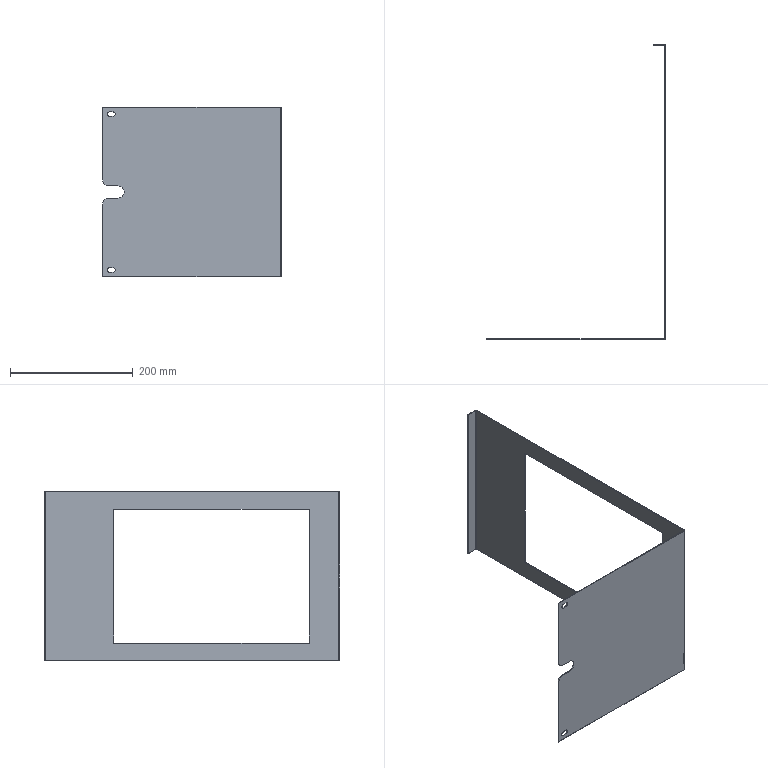Part | SolidWorks | features ICE 2, Cut 1, EdgeFlange 1, Fillet 1, FlatPattern 1, LPattern 1, SMBaseFlange 1, SheetMetal 1 | 1 solid | 40 faces | box 291.5 x 482 x 276.8 mm | volume 222164 mm3 | plane 29 | cylinder 11 | commonest cylinder face diameters 7 x4 20 x3 0.4 x2 3.4 x2
STEP:
#1=CARTESIAN_POINT('',(0.,0.,138.4));
#2=VERTEX_POINT('',#1);
#3=CARTESIAN_POINT('',(0.,0.,20.));
#4=VERTEX_POINT('',#3);
#5=CARTESIAN_POINT('',(0.,0.,138.4));
#6=DIRECTION('',(0.,0.,-1.));
#7=VECTOR('',#6,1000.);
#8=LINE('',#5,#7);
#9=EDGE_CURVE('',#2,#4,#8,.T.);
#10=ORIENTED_EDGE('',*,*,#9,.T.);
#11=CARTESIAN_POINT('',(0.,-1.5,20.));
#12=VERTEX_POINT('',#11);
#13=CARTESIAN_POINT('',(0.,-1.5,20.));
#14=DIRECTION('',(0.,-1.,0.));
#15=VECTOR('',#14,1000.);
#16=LINE('',#13,#15);
#17=EDGE_CURVE('',#4,#12,#16,.T.);
#18=ORIENTED_EDGE('',*,*,#17,.T.);
#19=CARTESIAN_POINT('',(0.,-1.5,138.4));
#20=VERTEX_POINT('',#19);
#21=CARTESIAN_POINT('',(0.,-1.5,138.4));
#22=DIRECTION('',(0.,0.,-1.));
#23=VECTOR('',#22,1000.);
#24=LINE('',#21,#23);
#25=EDGE_CURVE('',#20,#12,#24,.T.);
#26=ORIENTED_EDGE('',*,*,#25,.F.);
#27=CARTESIAN_POINT('',(0.,-1.5,138.4));
#28=DIRECTION('',(0.,1.,0.));
#29=VECTOR('',#28,1000.);
#30=LINE('',#27,#29);
#31=EDGE_CURVE('',#20,#2,#30,.T.);
#32=ORIENTED_EDGE('',*,*,#31,.T.);
#33=EDGE_LOOP('',(#10,#18,#26,#32));
#34=FACE_OUTER_BOUND('',#33,.T.);
#35=CARTESIAN_POINT('',(0.,-1.5,138.4));
#36=DIRECTION('',(-1.,0.,0.));
#37=DIRECTION('',(0.,0.,1.));
#38=AXIS2_PLACEMENT_3D('',#35,#36,#37);
#39=PLANE('',#38);
#40=ADVANCED_FACE('',(#34),#39,.T.);
#41=CARTESIAN_POINT('',(291.5,48.5,109.15));
#42=VERTEX_POINT('',#41);
#43=CARTESIAN_POINT('',(291.5,48.5,-109.35));
#44=VERTEX_POINT('',#43);
#45=CARTESIAN_POINT('',(291.5,48.5,109.15));
#46=DIRECTION('',(0.,0.,-1.));
#47=VECTOR('',#46,1000.);
#48=LINE('',#45,#47);
#49=EDGE_CURVE('',#42,#44,#48,.T.);
#50=ORIENTED_EDGE('',*,*,#49,.F.);
#51=CARTESIAN_POINT('',(291.5,367.1,109.15));
#52=VERTEX_POINT('',#51);
#53=CARTESIAN_POINT('',(291.5,367.1,109.15));
#54=DIRECTION('',(0.,-1.,0.));
#55=VECTOR('',#54,1000.);
#56=LINE('',#53,#55);
#57=EDGE_CURVE('',#52,#42,#56,.T.);
#58=ORIENTED_EDGE('',*,*,#57,.F.);
#59=CARTESIAN_POINT('',(291.5,367.1,-109.35));
#60=VERTEX_POINT('',#59);
#61=CARTESIAN_POINT('',(291.5,367.1,109.15));
#62=DIRECTION('',(0.,0.,1.));
#63=VECTOR('',#62,1000.);
#64=LINE('',#61,#63);
#65=EDGE_CURVE('',#60,#52,#64,.T.);
#66=ORIENTED_EDGE('',*,*,#65,.F.);
#67=CARTESIAN_POINT('',(291.5,367.1,-109.35));
#68=DIRECTION('',(0.,1.,0.));
#69=VECTOR('',#68,1000.);
#70=LINE('',#67,#69);
#71=EDGE_CURVE('',#44,#60,#70,.T.);
#72=ORIENTED_EDGE('',*,*,#71,.F.);
#73=EDGE_LOOP('',(#50,#58,#66,#72));
#74=FACE_BOUND('',#73,.T.);
#75=CARTESIAN_POINT('',(291.5,478.8,-138.4));
#76=VERTEX_POINT('',#75);
#77=CARTESIAN_POINT('',(291.5,478.8,138.4));
#78=VERTEX_POINT('',#77);
#79=CARTESIAN_POINT('',(291.5,478.8,-138.4));
#80=DIRECTION('',(0.,0.,1.));
#81=VECTOR('',#80,1000.);
#82=LINE('',#79,#81);
#83=EDGE_CURVE('',#76,#78,#82,.T.);
#84=ORIENTED_EDGE('',*,*,#83,.T.);
#85=CARTESIAN_POINT('',(291.5,0.2,138.4));
#86=VERTEX_POINT('',#85);
#87=CARTESIAN_POINT('',(291.5,0.,138.4));
#88=DIRECTION('',(0.,1.,0.));
#89=VECTOR('',#88,1000.);
#90=LINE('',#87,#89);
#91=EDGE_CURVE('',#86,#78,#90,.T.);
#92=ORIENTED_EDGE('',*,*,#91,.F.);
#93=CARTESIAN_POINT('',(291.5,0.2,-138.4));
#94=VERTEX_POINT('',#93);
#95=CARTESIAN_POINT('',(291.5,0.2,138.4));
#96=DIRECTION('',(0.,0.,-1.));
#97=VECTOR('',#96,1000.);
#98=LINE('',#95,#97);
#99=EDGE_CURVE('',#86,#94,#98,.T.);
#100=ORIENTED_EDGE('',*,*,#99,.T.);
#101=CARTESIAN_POINT('',(291.5,0.,-138.4));
#102=DIRECTION('',(0.,1.,0.));
#103=VECTOR('',#102,1000.);
#104=LINE('',#101,#103);
#105=EDGE_CURVE('',#94,#76,#104,.T.);
#106=ORIENTED_EDGE('',*,*,#105,.T.);
#107=EDGE_LOOP('',(#84,#92,#100,#106));
#108=FACE_OUTER_BOUND('',#107,.T.);
#109=CARTESIAN_POINT('',(291.5,0.,138.4));
#110=DIRECTION('',(-1.,0.,0.));
#111=DIRECTION('',(0.,0.,1.));
#112=AXIS2_PLACEMENT_3D('',#109,#110,#111);
#113=PLANE('',#112);
#114=ADVANCED_FACE('',(#74,#108),#113,.F.);
#115=CARTESIAN_POINT('',(290.,367.1,109.15));
#116=VERTEX_POINT('',#115);
#117=CARTESIAN_POINT('',(290.,48.5,109.15));
#118=VERTEX_POINT('',#117);
#119=CARTESIAN_POINT('',(290.,367.1,109.15));
#120=DIRECTION('',(0.,-1.,0.));
#121=VECTOR('',#120,1000.);
#122=LINE('',#119,#121);
#123=EDGE_CURVE('',#116,#118,#122,.T.);
#124=ORIENTED_EDGE('',*,*,#123,.T.);
#125=CARTESIAN_POINT('',(290.,48.5,-109.35));
#126=VERTEX_POINT('',#125);
#127=CARTESIAN_POINT('',(290.,48.5,109.15));
#128=DIRECTION('',(0.,0.,-1.));
#129=VECTOR('',#128,1000.);
#130=LINE('',#127,#129);
#131=EDGE_CURVE('',#118,#126,#130,.T.);
#132=ORIENTED_EDGE('',*,*,#131,.T.);
#133=CARTESIAN_POINT('',(290.,367.1,-109.35));
#134=VERTEX_POINT('',#133);
#135=CARTESIAN_POINT('',(290.,367.1,-109.35));
#136=DIRECTION('',(0.,1.,0.));
#137=VECTOR('',#136,1000.);
#138=LINE('',#135,#137);
#139=EDGE_CURVE('',#126,#134,#138,.T.);
#140=ORIENTED_EDGE('',*,*,#139,.T.);
#141=CARTESIAN_POINT('',(290.,367.1,109.15));
#142=DIRECTION('',(0.,0.,1.));
#143=VECTOR('',#142,1000.);
#144=LINE('',#141,#143);
#145=EDGE_CURVE('',#134,#116,#144,.T.);
#146=ORIENTED_EDGE('',*,*,#145,.T.);
#147=EDGE_LOOP('',(#124,#132,#140,#146));
#148=FACE_BOUND('',#147,.T.);
#149=CARTESIAN_POINT('',(290.,0.2,138.4));
#150=VERTEX_POINT('',#149);
#151=CARTESIAN_POINT('',(290.,478.8,138.4));
#152=VERTEX_POINT('',#151);
#153=CARTESIAN_POINT('',(290.,0.,138.4));
#154=DIRECTION('',(0.,1.,0.));
#155=VECTOR('',#154,1000.);
#156=LINE('',#153,#155);
#157=EDGE_CURVE('',#150,#152,#156,.T.);
#158=ORIENTED_EDGE('',*,*,#157,.T.);
#159=CARTESIAN_POINT('',(290.,478.8,-138.4));
#160=VERTEX_POINT('',#159);
#161=CARTESIAN_POINT('',(290.,478.8,-138.4));
#162=DIRECTION('',(0.,0.,1.));
#163=VECTOR('',#162,1000.);
#164=LINE('',#161,#163);
#165=EDGE_CURVE('',#160,#152,#164,.T.);
#166=ORIENTED_EDGE('',*,*,#165,.F.);
#167=CARTESIAN_POINT('',(290.,0.2,-138.4));
#168=VERTEX_POINT('',#167);
#169=CARTESIAN_POINT('',(290.,0.,-138.4));
#170=DIRECTION('',(0.,1.,0.));
#171=VECTOR('',#170,1000.);
#172=LINE('',#169,#171);
#173=EDGE_CURVE('',#168,#160,#172,.T.);
#174=ORIENTED_EDGE('',*,*,#173,.F.);
#175=CARTESIAN_POINT('',(290.,0.2,138.4));
#176=DIRECTION('',(0.,0.,-1.));
#177=VECTOR('',#176,1000.);
#178=LINE('',#175,#177);
#179=EDGE_CURVE('',#150,#168,#178,.T.);
#180=ORIENTED_EDGE('',*,*,#179,.F.);
#181=EDGE_LOOP('',(#158,#166,#174,#180));
#182=FACE_OUTER_BOUND('',#181,.T.);
#183=CARTESIAN_POINT('',(290.,0.,138.4));
#184=DIRECTION('',(-1.,0.,0.));
#185=DIRECTION('',(0.,0.,1.));
#186=AXIS2_PLACEMENT_3D('',#183,#184,#185);
#187=PLANE('',#186);
#188=ADVANCED_FACE('',(#148,#182),#187,.T.);
#189=ORIENTED_EDGE('',*,*,#173,.T.);
#190=CARTESIAN_POINT('',(290.,478.8,-138.4));
#191=DIRECTION('',(1.,0.,0.));
#192=VECTOR('',#191,1000.);
#193=LINE('',#190,#192);
#194=EDGE_CURVE('',#160,#76,#193,.T.);
#195=ORIENTED_EDGE('',*,*,#194,.T.);
#196=ORIENTED_EDGE('',*,*,#105,.F.);
#197=CARTESIAN_POINT('',(291.5,0.2,-138.4));
#198=DIRECTION('',(-1.,0.,0.));
#199=VECTOR('',#198,1000.);
#200=LINE('',#197,#199);
#201=EDGE_CURVE('',#94,#168,#200,.T.);
#202=ORIENTED_EDGE('',*,*,#201,.T.);
#203=EDGE_LOOP('',(#189,#195,#196,#202));
#204=FACE_OUTER_BOUND('',#203,.T.);
#205=CARTESIAN_POINT('',(289.8,0.2,-138.4));
#206=DIRECTION('',(0.,0.,-1.));
#207=DIRECTION('',(-1.,0.,0.));
#208=AXIS2_PLACEMENT_3D('',#205,#206,#207);
#209=PLANE('',#208);
#210=ADVANCED_FACE('',(#204),#209,.T.);
#211=CARTESIAN_POINT('',(290.,0.2,138.4));
#212=DIRECTION('',(1.,0.,0.));
#213=VECTOR('',#212,1000.);
#214=LINE('',#211,#213);
#215=EDGE_CURVE('',#150,#86,#214,.T.);
#216=ORIENTED_EDGE('',*,*,#215,.F.);
#217=CARTESIAN_POINT('',(289.8,0.,138.4));
#218=VERTEX_POINT('',#217);
#219=CARTESIAN_POINT('',(289.8,0.2,138.4));
#220=DIRECTION('',(0.,0.,1.));
#221=DIRECTION('',(-1.,0.,0.));
#222=AXIS2_PLACEMENT_3D('',#219,#220,#221);
#223=CIRCLE('',#222,0.2);
#224=EDGE_CURVE('',#218,#150,#223,.T.);
#225=ORIENTED_EDGE('',*,*,#224,.F.);
#226=CARTESIAN_POINT('',(289.8,-1.5,138.4));
#227=VERTEX_POINT('',#226);
#228=CARTESIAN_POINT('',(289.8,-1.5,138.4));
#229=DIRECTION('',(0.,1.,0.));
#230=VECTOR('',#229,1000.);
#231=LINE('',#228,#230);
#232=EDGE_CURVE('',#227,#218,#231,.T.);
#233=ORIENTED_EDGE('',*,*,#232,.F.);
#234=CARTESIAN_POINT('',(289.8,0.2,138.4));
#235=DIRECTION('',(0.,0.,1.));
#236=DIRECTION('',(1.,0.,0.));
#237=AXIS2_PLACEMENT_3D('',#234,#235,#236);
#238=CIRCLE('',#237,1.7);
#239=EDGE_CURVE('',#227,#86,#238,.T.);
#240=ORIENTED_EDGE('',*,*,#239,.T.);
#241=EDGE_LOOP('',(#216,#225,#233,#240));
#242=FACE_OUTER_BOUND('',#241,.T.);
#243=CARTESIAN_POINT('',(290.,0.2,138.4));
#244=DIRECTION('',(0.,0.,1.));
#245=DIRECTION('',(1.,0.,0.));
#246=AXIS2_PLACEMENT_3D('',#243,#244,#245);
#247=PLANE('',#246);
#248=ADVANCED_FACE('',(#242),#247,.T.);
#249=CARTESIAN_POINT('',(290.,478.8,138.4));
#250=DIRECTION('',(1.,0.,0.));
#251=VECTOR('',#250,1000.);
#252=LINE('',#249,#251);
#253=EDGE_CURVE('',#152,#78,#252,.T.);
#254=ORIENTED_EDGE('',*,*,#253,.F.);
#255=ORIENTED_EDGE('',*,*,#157,.F.);
#256=ORIENTED_EDGE('',*,*,#215,.T.);
#257=ORIENTED_EDGE('',*,*,#91,.T.);
#258=EDGE_LOOP('',(#254,#255,#256,#257));
#259=FACE_OUTER_BOUND('',#258,.T.);
#260=CARTESIAN_POINT('',(289.8,-1.5,138.4));
#261=DIRECTION('',(0.,0.,1.));
#262=DIRECTION('',(1.,0.,0.));
#263=AXIS2_PLACEMENT_3D('',#260,#261,#262);
#264=PLANE('',#263);
#265=ADVANCED_FACE('',(#259),#264,.T.);
#266=CARTESIAN_POINT('',(289.8,0.,-138.4));
#267=VERTEX_POINT('',#266);
#268=CARTESIAN_POINT('',(289.8,-1.5,-138.4));
#269=VERTEX_POINT('',#268);
#270=CARTESIAN_POINT('',(289.8,0.,-138.4));
#271=DIRECTION('',(0.,-1.,0.));
#272=VECTOR('',#271,1000.);
#273=LINE('',#270,#272);
#274=EDGE_CURVE('',#267,#269,#273,.T.);
#275=ORIENTED_EDGE('',*,*,#274,.F.);
#276=CARTESIAN_POINT('',(289.8,0.2,-138.4));
#277=DIRECTION('',(0.,0.,1.));
#278=DIRECTION('',(-1.,0.,0.));
#279=AXIS2_PLACEMENT_3D('',#276,#277,#278);
#280=CIRCLE('',#279,0.2);
#281=EDGE_CURVE('',#267,#168,#280,.T.);
#282=ORIENTED_EDGE('',*,*,#281,.T.);
#283=ORIENTED_EDGE('',*,*,#201,.F.);
#284=CARTESIAN_POINT('',(289.8,0.2,-138.4));
#285=DIRECTION('',(0.,0.,1.));
#286=DIRECTION('',(1.,0.,0.));
#287=AXIS2_PLACEMENT_3D('',#284,#285,#286);
#288=CIRCLE('',#287,1.7);
#289=EDGE_CURVE('',#269,#94,#288,.T.);
#290=ORIENTED_EDGE('',*,*,#289,.F.);
#291=EDGE_LOOP('',(#275,#282,#283,#290));
#292=FACE_OUTER_BOUND('',#291,.T.);
#293=CARTESIAN_POINT('',(289.8,0.,-138.4));
#294=DIRECTION('',(0.,0.,-1.));
#295=DIRECTION('',(-1.,0.,0.));
#296=AXIS2_PLACEMENT_3D('',#293,#294,#295);
#297=PLANE('',#296);
#298=ADVANCED_FACE('',(#292),#297,.T.);
#299=CARTESIAN_POINT('',(0.,0.,-138.4));
#300=VERTEX_POINT('',#299);
#301=CARTESIAN_POINT('',(0.,0.,-138.4));
#302=DIRECTION('',(1.,0.,0.));
#303=VECTOR('',#302,1000.);
#304=LINE('',#301,#303);
#305=EDGE_CURVE('',#300,#267,#304,.T.);
#306=ORIENTED_EDGE('',*,*,#305,.T.);
#307=ORIENTED_EDGE('',*,*,#274,.T.);
#308=CARTESIAN_POINT('',(0.,-1.5,-138.4));
#309=VERTEX_POINT('',#308);
#310=CARTESIAN_POINT('',(0.,-1.5,-138.4));
#311=DIRECTION('',(1.,0.,0.));
#312=VECTOR('',#311,1000.);
#313=LINE('',#310,#312);
#314=EDGE_CURVE('',#309,#269,#313,.T.);
#315=ORIENTED_EDGE('',*,*,#314,.F.);
#316=CARTESIAN_POINT('',(0.,-1.5,-138.4));
#317=DIRECTION('',(0.,1.,0.));
#318=VECTOR('',#317,1000.);
#319=LINE('',#316,#318);
#320=EDGE_CURVE('',#309,#300,#319,.T.);
#321=ORIENTED_EDGE('',*,*,#320,.T.);
#322=EDGE_LOOP('',(#306,#307,#315,#321));
#323=FACE_OUTER_BOUND('',#322,.T.);
#324=CARTESIAN_POINT('',(291.5,0.2,-138.4));
#325=DIRECTION('',(0.,0.,-1.));
#326=DIRECTION('',(-1.,0.,0.));
#327=AXIS2_PLACEMENT_3D('',#324,#325,#326);
#328=PLANE('',#327);
#329=ADVANCED_FACE('',(#323),#328,.T.);
#330=ORIENTED_EDGE('',*,*,#281,.F.);
#331=CARTESIAN_POINT('',(289.8,0.,138.4));
#332=DIRECTION('',(0.,0.,-1.));
#333=VECTOR('',#332,1000.);
#334=LINE('',#331,#333);
#335=EDGE_CURVE('',#218,#267,#334,.T.);
#336=ORIENTED_EDGE('',*,*,#335,.F.);
#337=ORIENTED_EDGE('',*,*,#224,.T.);
#338=ORIENTED_EDGE('',*,*,#179,.T.);
#339=EDGE_LOOP('',(#330,#336,#337,#338));
#340=FACE_OUTER_BOUND('',#339,.T.);
#341=CARTESIAN_POINT('',(289.8,0.2,138.4));
#342=DIRECTION('',(0.,0.,-1.));
#343=DIRECTION('',(-1.,0.,0.));
#344=AXIS2_PLACEMENT_3D('',#341,#342,#343);
#345=CYLINDRICAL_SURFACE('',#344,0.2);
#346=ADVANCED_FACE('',(#340),#345,.F.);
#347=CARTESIAN_POINT('',(10.,0.,10.));
#348=VERTEX_POINT('',#347);
#349=CARTESIAN_POINT('',(25.,0.,10.));
#350=VERTEX_POINT('',#349);
#351=CARTESIAN_POINT('',(25.,0.,10.));
#352=DIRECTION('',(1.,0.,0.));
#353=VECTOR('',#352,1000.);
#354=LINE('',#351,#353);
#355=EDGE_CURVE('',#348,#350,#354,.T.);
#356=ORIENTED_EDGE('',*,*,#355,.F.);
#357=CARTESIAN_POINT('',(10.,0.,20.));
#358=DIRECTION('',(0.,1.,0.));
#359=DIRECTION('',(0.,0.,1.));
#360=AXIS2_PLACEMENT_3D('',#357,#358,#359);
#361=CIRCLE('',#360,10.);
#362=EDGE_CURVE('',#348,#4,#361,.T.);
#363=ORIENTED_EDGE('',*,*,#362,.T.);
#364=ORIENTED_EDGE('',*,*,#9,.F.);
#365=CARTESIAN_POINT('',(0.,0.,138.4));
#366=DIRECTION('',(1.,0.,0.));
#367=VECTOR('',#366,1000.);
#368=LINE('',#365,#367);
#369=EDGE_CURVE('',#2,#218,#368,.T.);
#370=ORIENTED_EDGE('',*,*,#369,.T.);
#371=ORIENTED_EDGE('',*,*,#335,.T.);
#372=ORIENTED_EDGE('',*,*,#305,.F.);
#373=CARTESIAN_POINT('',(0.,0.,-20.));
#374=VERTEX_POINT('',#373);
#375=CARTESIAN_POINT('',(0.,0.,138.4));
#376=DIRECTION('',(0.,0.,-1.));
#377=VECTOR('',#376,1000.);
#378=LINE('',#375,#377);
#379=EDGE_CURVE('',#374,#300,#378,.T.);
#380=ORIENTED_EDGE('',*,*,#379,.F.);
#381=CARTESIAN_POINT('',(10.,0.,-10.));
#382=VERTEX_POINT('',#381);
#383=CARTESIAN_POINT('',(10.,0.,-20.));
#384=DIRECTION('',(0.,1.,0.));
#385=DIRECTION('',(0.,0.,1.));
#386=AXIS2_PLACEMENT_3D('',#383,#384,#385);
#387=CIRCLE('',#386,10.);
#388=EDGE_CURVE('',#374,#382,#387,.T.);
#389=ORIENTED_EDGE('',*,*,#388,.T.);
#390=CARTESIAN_POINT('',(25.,0.,-10.));
#391=VERTEX_POINT('',#390);
#392=CARTESIAN_POINT('',(25.,0.,-10.));
#393=DIRECTION('',(-1.,0.,0.));
#394=VECTOR('',#393,1000.);
#395=LINE('',#392,#394);
#396=EDGE_CURVE('',#391,#382,#395,.T.);
#397=ORIENTED_EDGE('',*,*,#396,.F.);
#398=CARTESIAN_POINT('',(25.,0.,0.));
#399=DIRECTION('',(0.,1.,0.));
#400=DIRECTION('',(0.,0.,1.));
#401=AXIS2_PLACEMENT_3D('',#398,#399,#400);
#402=CIRCLE('',#401,10.);
#403=EDGE_CURVE('',#350,#391,#402,.T.);
#404=ORIENTED_EDGE('',*,*,#403,.F.);
#405=EDGE_LOOP('',(#356,#363,#364,#370,#371,#372,#380,#389,#397,#404));
#406=FACE_OUTER_BOUND('',#405,.T.);
#407=CARTESIAN_POINT('',(11.,0.,-130.75));
#408=VERTEX_POINT('',#407);
#409=CARTESIAN_POINT('',(11.,0.,-123.75));
#410=VERTEX_POINT('',#409);
#411=CARTESIAN_POINT('',(11.,0.,-127.25));
#412=DIRECTION('',(0.,1.,0.));
#413=DIRECTION('',(0.,0.,1.));
#414=AXIS2_PLACEMENT_3D('',#411,#412,#413);
#415=CIRCLE('',#414,3.5);
#416=EDGE_CURVE('',#408,#410,#415,.T.);
#417=ORIENTED_EDGE('',*,*,#416,.F.);
#418=CARTESIAN_POINT('',(17.,0.,-130.75));
#419=VERTEX_POINT('',#418);
#420=CARTESIAN_POINT('',(11.,0.,-130.75));
#421=DIRECTION('',(-1.,0.,0.));
#422=VECTOR('',#421,1000.);
#423=LINE('',#420,#422);
#424=EDGE_CURVE('',#419,#408,#423,.T.);
#425=ORIENTED_EDGE('',*,*,#424,.F.);
#426=CARTESIAN_POINT('',(17.,0.,-123.75));
#427=VERTEX_POINT('',#426);
#428=CARTESIAN_POINT('',(17.,0.,-127.25));
#429=DIRECTION('',(0.,1.,0.));
#430=DIRECTION('',(0.,0.,1.));
#431=AXIS2_PLACEMENT_3D('',#428,#429,#430);
#432=CIRCLE('',#431,3.5);
#433=EDGE_CURVE('',#427,#419,#432,.T.);
#434=ORIENTED_EDGE('',*,*,#433,.F.);
#435=CARTESIAN_POINT('',(11.,0.,-123.75));
#436=DIRECTION('',(1.,0.,0.));
#437=VECTOR('',#436,1000.);
#438=LINE('',#435,#437);
#439=EDGE_CURVE('',#410,#427,#438,.T.);
#440=ORIENTED_EDGE('',*,*,#439,.F.);
#441=EDGE_LOOP('',(#417,#425,#434,#440));
#442=FACE_BOUND('',#441,.T.);
#443=CARTESIAN_POINT('',(11.,0.,123.55));
#444=VERTEX_POINT('',#443);
#445=CARTESIAN_POINT('',(11.,0.,130.55));
#446=VERTEX_POINT('',#445);
#447=CARTESIAN_POINT('',(11.,0.,127.05));
#448=DIRECTION('',(0.,1.,0.));
#449=DIRECTION('',(0.,0.,1.));
#450=AXIS2_PLACEMENT_3D('',#447,#448,#449);
#451=CIRCLE('',#450,3.5);
#452=EDGE_CURVE('',#444,#446,#451,.T.);
#453=ORIENTED_EDGE('',*,*,#452,.F.);
#454=CARTESIAN_POINT('',(17.,0.,123.55));
#455=VERTEX_POINT('',#454);
#456=CARTESIAN_POINT('',(11.,0.,123.55));
#457=DIRECTION('',(-1.,0.,0.));
#458=VECTOR('',#457,1000.);
#459=LINE('',#456,#458);
#460=EDGE_CURVE('',#455,#444,#459,.T.);
#461=ORIENTED_EDGE('',*,*,#460,.F.);
#462=CARTESIAN_POINT('',(17.,0.,130.55));
#463=VERTEX_POINT('',#462);
#464=CARTESIAN_POINT('',(17.,0.,127.05));
#465=DIRECTION('',(0.,1.,0.));
#466=DIRECTION('',(0.,0.,1.));
#467=AXIS2_PLACEMENT_3D('',#464,#465,#466);
#468=CIRCLE('',#467,3.5);
#469=EDGE_CURVE('',#463,#455,#468,.T.);
#470=ORIENTED_EDGE('',*,*,#469,.F.);
#471=CARTESIAN_POINT('',(11.,0.,130.55));
#472=DIRECTION('',(1.,0.,0.));
#473=VECTOR('',#472,1000.);
#474=LINE('',#471,#473);
#475=EDGE_CURVE('',#446,#463,#474,.T.);
#476=ORIENTED_EDGE('',*,*,#475,.F.);
#477=EDGE_LOOP('',(#453,#461,#470,#476));
#478=FACE_BOUND('',#477,.T.);
#479=CARTESIAN_POINT('',(0.,0.,138.4));
#480=DIRECTION('',(0.,1.,0.));
#481=DIRECTION('',(0.,0.,1.));
#482=AXIS2_PLACEMENT_3D('',#479,#480,#481);
#483=PLANE('',#482);
#484=ADVANCED_FACE('',(#406,#442,#478),#483,.T.);
#485=CARTESIAN_POINT('',(0.,-1.5,-20.));
#486=VERTEX_POINT('',#485);
#487=CARTESIAN_POINT('',(0.,-1.5,138.4));
#488=DIRECTION('',(0.,0.,-1.));
#489=VECTOR('',#488,1000.);
#490=LINE('',#487,#489);
#491=EDGE_CURVE('',#486,#309,#490,.T.);
#492=ORIENTED_EDGE('',*,*,#491,.F.);
#493=CARTESIAN_POINT('',(0.,0.,-20.));
#494=DIRECTION('',(0.,1.,0.));
#495=VECTOR('',#494,1000.);
#496=LINE('',#493,#495);
#497=EDGE_CURVE('',#486,#374,#496,.T.);
#498=ORIENTED_EDGE('',*,*,#497,.T.);
#499=ORIENTED_EDGE('',*,*,#379,.T.);
#500=ORIENTED_EDGE('',*,*,#320,.F.);
#501=EDGE_LOOP('',(#492,#498,#499,#500));
#502=FACE_OUTER_BOUND('',#501,.T.);
#503=CARTESIAN_POINT('',(0.,-1.5,138.4));
#504=DIRECTION('',(-1.,0.,0.));
#505=DIRECTION('',(0.,0.,1.));
#506=AXIS2_PLACEMENT_3D('',#503,#504,#505);
#507=PLANE('',#506);
#508=ADVANCED_FACE('',(#502),#507,.T.);
#509=CARTESIAN_POINT('',(17.,-1.5,-130.75));
#510=VERTEX_POINT('',#509);
#511=CARTESIAN_POINT('',(11.,-1.5,-130.75));
#512=VERTEX_POINT('',#511);
#513=CARTESIAN_POINT('',(11.,-1.5,-130.75));
#514=DIRECTION('',(-1.,0.,0.));
#515=VECTOR('',#514,1000.);
#516=LINE('',#513,#515);
#517=EDGE_CURVE('',#510,#512,#516,.T.);
#518=ORIENTED_EDGE('',*,*,#517,.T.);
#519=CARTESIAN_POINT('',(11.,-1.5,-123.75));
#520=VERTEX_POINT('',#519);
#521=CARTESIAN_POINT('',(11.,-1.5,-127.25));
#522=DIRECTION('',(0.,1.,0.));
#523=DIRECTION('',(0.,0.,1.));
#524=AXIS2_PLACEMENT_3D('',#521,#522,#523);
#525=CIRCLE('',#524,3.5);
#526=EDGE_CURVE('',#512,#520,#525,.T.);
#527=ORIENTED_EDGE('',*,*,#526,.T.);
#528=CARTESIAN_POINT('',(17.,-1.5,-123.75));
#529=VERTEX_POINT('',#528);
#530=CARTESIAN_POINT('',(11.,-1.5,-123.75));
#531=DIRECTION('',(1.,0.,0.));
#532=VECTOR('',#531,1000.);
#533=LINE('',#530,#532);
#534=EDGE_CURVE('',#520,#529,#533,.T.);
#535=ORIENTED_EDGE('',*,*,#534,.T.);
#536=CARTESIAN_POINT('',(17.,-1.5,-127.25));
#537=DIRECTION('',(0.,1.,0.));
#538=DIRECTION('',(0.,0.,1.));
#539=AXIS2_PLACEMENT_3D('',#536,#537,#538);
#540=CIRCLE('',#539,3.5);
#541=EDGE_CURVE('',#529,#510,#540,.T.);
#542=ORIENTED_EDGE('',*,*,#541,.T.);
#543=EDGE_LOOP('',(#518,#527,#535,#542));
#544=FACE_BOUND('',#543,.T.);
#545=CARTESIAN_POINT('',(17.,-1.5,123.55));
#546=VERTEX_POINT('',#545);
#547=CARTESIAN_POINT('',(11.,-1.5,123.55));
#548=VERTEX_POINT('',#547);
#549=CARTESIAN_POINT('',(11.,-1.5,123.55));
#550=DIRECTION('',(-1.,0.,0.));
#551=VECTOR('',#550,1000.);
#552=LINE('',#549,#551);
#553=EDGE_CURVE('',#546,#548,#552,.T.);
#554=ORIENTED_EDGE('',*,*,#553,.T.);
#555=CARTESIAN_POINT('',(11.,-1.5,130.55));
#556=VERTEX_POINT('',#555);
#557=CARTESIAN_POINT('',(11.,-1.5,127.05));
#558=DIRECTION('',(0.,1.,0.));
#559=DIRECTION('',(0.,0.,1.));
#560=AXIS2_PLACEMENT_3D('',#557,#558,#559);
#561=CIRCLE('',#560,3.5);
#562=EDGE_CURVE('',#548,#556,#561,.T.);
#563=ORIENTED_EDGE('',*,*,#562,.T.);
#564=CARTESIAN_POINT('',(17.,-1.5,130.55));
#565=VERTEX_POINT('',#564);
#566=CARTESIAN_POINT('',(11.,-1.5,130.55));
#567=DIRECTION('',(1.,0.,0.));
#568=VECTOR('',#567,1000.);
#569=LINE('',#566,#568);
#570=EDGE_CURVE('',#556,#565,#569,.T.);
#571=ORIENTED_EDGE('',*,*,#570,.T.);
#572=CARTESIAN_POINT('',(17.,-1.5,127.05));
#573=DIRECTION('',(0.,1.,0.));
#574=DIRECTION('',(0.,0.,1.));
#575=AXIS2_PLACEMENT_3D('',#572,#573,#574);
#576=CIRCLE('',#575,3.5);
#577=EDGE_CURVE('',#565,#546,#576,.T.);
#578=ORIENTED_EDGE('',*,*,#577,.T.);
#579=EDGE_LOOP('',(#554,#563,#571,#578));
#580=FACE_BOUND('',#579,.T.);
#581=ORIENTED_EDGE('',*,*,#25,.T.);
#582=CARTESIAN_POINT('',(10.,-1.5,10.));
#583=VERTEX_POINT('',#582);
#584=CARTESIAN_POINT('',(10.,-1.5,20.));
#585=DIRECTION('',(0.,-1.,0.));
#586=DIRECTION('',(0.,0.,1.));
#587=AXIS2_PLACEMENT_3D('',#584,#585,#586);
#588=CIRCLE('',#587,10.);
#589=EDGE_CURVE('',#12,#583,#588,.T.);
#590=ORIENTED_EDGE('',*,*,#589,.T.);
#591=CARTESIAN_POINT('',(25.,-1.5,10.));
#592=VERTEX_POINT('',#591);
#593=CARTESIAN_POINT('',(25.,-1.5,10.));
#594=DIRECTION('',(1.,0.,0.));
#595=VECTOR('',#594,1000.);
#596=LINE('',#593,#595);
#597=EDGE_CURVE('',#583,#592,#596,.T.);
#598=ORIENTED_EDGE('',*,*,#597,.T.);
#599=CARTESIAN_POINT('',(25.,-1.5,-10.));
#600=VERTEX_POINT('',#599);
#601=CARTESIAN_POINT('',(25.,-1.5,0.));
#602=DIRECTION('',(0.,1.,0.));
#603=DIRECTION('',(0.,0.,1.));
#604=AXIS2_PLACEMENT_3D('',#601,#602,#603);
#605=CIRCLE('',#604,10.);
#606=EDGE_CURVE('',#592,#600,#605,.T.);
#607=ORIENTED_EDGE('',*,*,#606,.T.);
#608=CARTESIAN_POINT('',(10.,-1.5,-10.));
#609=VERTEX_POINT('',#608);
#610=CARTESIAN_POINT('',(25.,-1.5,-10.));
#611=DIRECTION('',(-1.,0.,0.));
#612=VECTOR('',#611,1000.);
#613=LINE('',#610,#612);
#614=EDGE_CURVE('',#600,#609,#613,.T.);
#615=ORIENTED_EDGE('',*,*,#614,.T.);
#616=CARTESIAN_POINT('',(10.,-1.5,-20.));
#617=DIRECTION('',(0.,-1.,0.));
#618=DIRECTION('',(0.,0.,1.));
#619=AXIS2_PLACEMENT_3D('',#616,#617,#618);
#620=CIRCLE('',#619,10.);
#621=EDGE_CURVE('',#609,#486,#620,.T.);
#622=ORIENTED_EDGE('',*,*,#621,.T.);
#623=ORIENTED_EDGE('',*,*,#491,.T.);
#624=ORIENTED_EDGE('',*,*,#314,.T.);
#625=CARTESIAN_POINT('',(289.8,-1.5,138.4));
#626=DIRECTION('',(0.,0.,-1.));
#627=VECTOR('',#626,1000.);
#628=LINE('',#625,#627);
#629=EDGE_CURVE('',#227,#269,#628,.T.);
#630=ORIENTED_EDGE('',*,*,#629,.F.);
#631=CARTESIAN_POINT('',(0.,-1.5,138.4));
#632=DIRECTION('',(1.,0.,0.));
#633=VECTOR('',#632,1000.);
#634=LINE('',#631,#633);
#635=EDGE_CURVE('',#20,#227,#634,.T.);
#636=ORIENTED_EDGE('',*,*,#635,.F.);
#637=EDGE_LOOP('',(#581,#590,#598,#607,#615,#622,#623,#624,#630,#636));
#638=FACE_OUTER_BOUND('',#637,.T.);
#639=CARTESIAN_POINT('',(0.,-1.5,138.4));
#640=DIRECTION('',(0.,1.,0.));
#641=DIRECTION('',(0.,0.,1.));
#642=AXIS2_PLACEMENT_3D('',#639,#640,#641);
#643=PLANE('',#642);
#644=ADVANCED_FACE('',(#544,#580,#638),#643,.F.);
#645=ORIENTED_EDGE('',*,*,#289,.T.);
#646=ORIENTED_EDGE('',*,*,#99,.F.);
#647=ORIENTED_EDGE('',*,*,#239,.F.);
#648=ORIENTED_EDGE('',*,*,#629,.T.);
#649=EDGE_LOOP('',(#645,#646,#647,#648));
#650=FACE_OUTER_BOUND('',#649,.T.);
#651=CARTESIAN_POINT('',(289.8,0.2,138.4));
#652=DIRECTION('',(0.,0.,-1.));
#653=DIRECTION('',(-1.,0.,0.));
#654=AXIS2_PLACEMENT_3D('',#651,#652,#653);
#655=CYLINDRICAL_SURFACE('',#654,1.7);
#656=ADVANCED_FACE('',(#650),#655,.T.);
#657=ORIENTED_EDGE('',*,*,#635,.T.);
#658=ORIENTED_EDGE('',*,*,#232,.T.);
#659=ORIENTED_EDGE('',*,*,#369,.F.);
#660=ORIENTED_EDGE('',*,*,#31,.F.);
#661=EDGE_LOOP('',(#657,#658,#659,#660));
#662=FACE_OUTER_BOUND('',#661,.T.);
#663=CARTESIAN_POINT('',(289.8,0.2,138.4));
#664=DIRECTION('',(0.,0.,-1.));
#665=DIRECTION('',(-1.,0.,0.));
#666=AXIS2_PLACEMENT_3D('',#663,#664,#665);
#667=PLANE('',#666);
#668=ADVANCED_FACE('',(#662),#667,.F.);
#669=CARTESIAN_POINT('',(289.8,479.,138.4));
#670=VERTEX_POINT('',#669);
#671=CARTESIAN_POINT('',(289.8,480.5,138.4));
#672=VERTEX_POINT('',#671);
#673=CARTESIAN_POINT('',(289.8,480.5,138.4));
#674=DIRECTION('',(0.,1.,0.));
#675=VECTOR('',#674,1000.);
#676=LINE('',#673,#675);
#677=EDGE_CURVE('',#670,#672,#676,.T.);
#678=ORIENTED_EDGE('',*,*,#677,.F.);
#679=CARTESIAN_POINT('',(289.8,478.8,138.4));
#680=DIRECTION('',(0.,0.,1.));
#681=DIRECTION('',(-1.,0.,0.));
#682=AXIS2_PLACEMENT_3D('',#679,#680,#681);
#683=CIRCLE('',#682,0.2);
#684=EDGE_CURVE('',#152,#670,#683,.T.);
#685=ORIENTED_EDGE('',*,*,#684,.F.);
#686=ORIENTED_EDGE('',*,*,#253,.T.);
#687=CARTESIAN_POINT('',(289.8,478.8,138.4));
#688=DIRECTION('',(0.,0.,1.));
#689=DIRECTION('',(-1.,0.,0.));
#690=AXIS2_PLACEMENT_3D('',#687,#688,#689);
#691=CIRCLE('',#690,1.7);
#692=EDGE_CURVE('',#78,#672,#691,.T.);
#693=ORIENTED_EDGE('',*,*,#692,.T.);
#694=EDGE_LOOP('',(#678,#685,#686,#693));
#695=FACE_OUTER_BOUND('',#694,.T.);
#696=CARTESIAN_POINT('',(289.8,478.8,138.4));
#697=DIRECTION('',(0.,0.,1.));
#698=DIRECTION('',(1.,0.,0.));
#699=AXIS2_PLACEMENT_3D('',#696,#697,#698);
#700=PLANE('',#699);
#701=ADVANCED_FACE('',(#695),#700,.T.);
#702=CARTESIAN_POINT('',(289.8,479.,-138.4));
#703=VERTEX_POINT('',#702);
#704=CARTESIAN_POINT('',(289.8,478.8,-138.4));
#705=DIRECTION('',(0.,0.,-1.));
#706=DIRECTION('',(-1.,0.,0.));
#707=AXIS2_PLACEMENT_3D('',#704,#705,#706);
#708=CIRCLE('',#707,0.2);
#709=EDGE_CURVE('',#703,#160,#708,.T.);
#710=ORIENTED_EDGE('',*,*,#709,.F.);
#711=CARTESIAN_POINT('',(289.8,480.5,-138.4));
#712=VERTEX_POINT('',#711);
#713=CARTESIAN_POINT('',(289.8,479.,-138.4));
#714=DIRECTION('',(0.,1.,0.));
#715=VECTOR('',#714,1000.);
#716=LINE('',#713,#715);
#717=EDGE_CURVE('',#703,#712,#716,.T.);
#718=ORIENTED_EDGE('',*,*,#717,.T.);
#719=CARTESIAN_POINT('',(289.8,478.8,-138.4));
#720=DIRECTION('',(0.,0.,-1.));
#721=DIRECTION('',(-1.,0.,0.));
#722=AXIS2_PLACEMENT_3D('',#719,#720,#721);
#723=CIRCLE('',#722,1.7);
#724=EDGE_CURVE('',#712,#76,#723,.T.);
#725=ORIENTED_EDGE('',*,*,#724,.T.);
#726=ORIENTED_EDGE('',*,*,#194,.F.);
#727=EDGE_LOOP('',(#710,#718,#725,#726));
#728=FACE_OUTER_BOUND('',#727,.T.);
#729=CARTESIAN_POINT('',(289.8,478.8,-138.4));
#730=DIRECTION('',(0.,0.,1.));
#731=DIRECTION('',(1.,0.,0.));
#732=AXIS2_PLACEMENT_3D('',#729,#730,#731);
#733=PLANE('',#732);
#734=ADVANCED_FACE('',(#728),#733,.F.);
#735=ORIENTED_EDGE('',*,*,#83,.F.);
#736=ORIENTED_EDGE('',*,*,#724,.F.);
#737=CARTESIAN_POINT('',(289.8,480.5,0.));
#738=DIRECTION('',(0.,0.,-1.));
#739=VECTOR('',#738,1000.);
#740=LINE('',#737,#739);
#741=EDGE_CURVE('',#672,#712,#740,.T.);
#742=ORIENTED_EDGE('',*,*,#741,.F.);
#743=ORIENTED_EDGE('',*,*,#692,.F.);
#744=EDGE_LOOP('',(#735,#736,#742,#743));
#745=FACE_OUTER_BOUND('',#744,.T.);
#746=CARTESIAN_POINT('',(289.8,478.8,-138.4));
#747=DIRECTION('',(0.,0.,-1.));
#748=DIRECTION('',(0.,1.,0.));
#749=AXIS2_PLACEMENT_3D('',#746,#747,#748);
#750=CYLINDRICAL_SURFACE('',#749,1.7);
#751=ADVANCED_FACE('',(#745),#750,.T.);
#752=ORIENTED_EDGE('',*,*,#165,.T.);
#753=ORIENTED_EDGE('',*,*,#684,.T.);
#754=CARTESIAN_POINT('',(289.8,479.,138.4));
#755=DIRECTION('',(0.,0.,-1.));
#756=VECTOR('',#755,1000.);
#757=LINE('',#754,#756);
#758=EDGE_CURVE('',#670,#703,#757,.T.);
#759=ORIENTED_EDGE('',*,*,#758,.T.);
#760=ORIENTED_EDGE('',*,*,#709,.T.);
#761=EDGE_LOOP('',(#752,#753,#759,#760));
#762=FACE_OUTER_BOUND('',#761,.T.);
#763=CARTESIAN_POINT('',(289.8,478.8,-138.4));
#764=DIRECTION('',(0.,0.,-1.));
#765=DIRECTION('',(0.,1.,0.));
#766=AXIS2_PLACEMENT_3D('',#763,#764,#765);
#767=CYLINDRICAL_SURFACE('',#766,0.2);
#768=ADVANCED_FACE('',(#762),#767,.F.);
#769=CARTESIAN_POINT('',(271.5,480.5,-138.4));
#770=VERTEX_POINT('',#769);
#771=CARTESIAN_POINT('',(290.,480.5,-138.4));
#772=DIRECTION('',(1.,0.,0.));
#773=VECTOR('',#772,1000.);
#774=LINE('',#771,#773);
#775=EDGE_CURVE('',#770,#712,#774,.T.);
#776=ORIENTED_EDGE('',*,*,#775,.T.);
#777=ORIENTED_EDGE('',*,*,#717,.F.);
#778=CARTESIAN_POINT('',(271.5,479.,-138.4));
#779=VERTEX_POINT('',#778);
#780=CARTESIAN_POINT('',(0.,479.,-138.4));
#781=DIRECTION('',(1.,0.,0.));
#782=VECTOR('',#781,1000.);
#783=LINE('',#780,#782);
#784=EDGE_CURVE('',#779,#703,#783,.T.);
#785=ORIENTED_EDGE('',*,*,#784,.F.);
#786=CARTESIAN_POINT('',(271.5,480.5,-138.4));
#787=DIRECTION('',(0.,-1.,0.));
#788=VECTOR('',#787,1000.);
#789=LINE('',#786,#788);
#790=EDGE_CURVE('',#770,#779,#789,.T.);
#791=ORIENTED_EDGE('',*,*,#790,.F.);
#792=EDGE_LOOP('',(#776,#777,#785,#791));
#793=FACE_OUTER_BOUND('',#792,.T.);
#794=CARTESIAN_POINT('',(290.,480.5,-138.4));
#795=DIRECTION('',(0.,0.,-1.));
#796=DIRECTION('',(-1.,0.,0.));
#797=AXIS2_PLACEMENT_3D('',#794,#795,#796);
#798=PLANE('',#797);
#799=ADVANCED_FACE('',(#793),#798,.T.);
#800=CARTESIAN_POINT('',(271.5,479.,138.4));
#801=VERTEX_POINT('',#800);
#802=CARTESIAN_POINT('',(0.,479.,138.4));
#803=DIRECTION('',(-1.,0.,0.));
#804=VECTOR('',#803,1000.);
#805=LINE('',#802,#804);
#806=EDGE_CURVE('',#670,#801,#805,.T.);
#807=ORIENTED_EDGE('',*,*,#806,.F.);
#808=ORIENTED_EDGE('',*,*,#677,.T.);
#809=CARTESIAN_POINT('',(271.5,480.5,138.4));
#810=VERTEX_POINT('',#809);
#811=CARTESIAN_POINT('',(271.5,480.5,138.4));
#812=DIRECTION('',(-1.,0.,0.));
#813=VECTOR('',#812,1000.);
#814=LINE('',#811,#813);
#815=EDGE_CURVE('',#672,#810,#814,.T.);
#816=ORIENTED_EDGE('',*,*,#815,.T.);
#817=CARTESIAN_POINT('',(271.5,480.5,138.4));
#818=DIRECTION('',(0.,-1.,0.));
#819=VECTOR('',#818,1000.);
#820=LINE('',#817,#819);
#821=EDGE_CURVE('',#810,#801,#820,.T.);
#822=ORIENTED_EDGE('',*,*,#821,.T.);
#823=EDGE_LOOP('',(#807,#808,#816,#822));
#824=FACE_OUTER_BOUND('',#823,.T.);
#825=CARTESIAN_POINT('',(271.5,480.5,138.4));
#826=DIRECTION('',(0.,0.,1.));
#827=DIRECTION('',(1.,0.,0.));
#828=AXIS2_PLACEMENT_3D('',#825,#826,#827);
#829=PLANE('',#828);
#830=ADVANCED_FACE('',(#824),#829,.T.);
#831=ORIENTED_EDGE('',*,*,#815,.F.);
#832=ORIENTED_EDGE('',*,*,#741,.T.);
#833=ORIENTED_EDGE('',*,*,#775,.F.);
#834=CARTESIAN_POINT('',(271.5,480.5,-138.4));
#835=DIRECTION('',(0.,0.,-1.));
#836=VECTOR('',#835,1000.);
#837=LINE('',#834,#836);
#838=EDGE_CURVE('',#810,#770,#837,.T.);
#839=ORIENTED_EDGE('',*,*,#838,.F.);
#840=EDGE_LOOP('',(#831,#832,#833,#839));
#841=FACE_OUTER_BOUND('',#840,.T.);
#842=CARTESIAN_POINT('',(0.,480.5,0.));
#843=DIRECTION('',(0.,1.,0.));
#844=DIRECTION('',(-1.,0.,0.));
#845=AXIS2_PLACEMENT_3D('',#842,#843,#844);
#846=PLANE('',#845);
#847=ADVANCED_FACE('',(#841),#846,.T.);
#848=ORIENTED_EDGE('',*,*,#758,.F.);
#849=ORIENTED_EDGE('',*,*,#806,.T.);
#850=CARTESIAN_POINT('',(271.5,479.,0.));
#851=DIRECTION('',(0.,0.,-1.));
#852=VECTOR('',#851,1000.);
#853=LINE('',#850,#852);
#854=EDGE_CURVE('',#801,#779,#853,.T.);
#855=ORIENTED_EDGE('',*,*,#854,.T.);
#856=ORIENTED_EDGE('',*,*,#784,.T.);
#857=EDGE_LOOP('',(#848,#849,#855,#856));
#858=FACE_OUTER_BOUND('',#857,.T.);
#859=CARTESIAN_POINT('',(0.,479.,0.));
#860=DIRECTION('',(0.,1.,0.));
#861=DIRECTION('',(-1.,0.,0.));
#862=AXIS2_PLACEMENT_3D('',#859,#860,#861);
#863=PLANE('',#862);
#864=ADVANCED_FACE('',(#858),#863,.F.);
#865=ORIENTED_EDGE('',*,*,#854,.F.);
#866=ORIENTED_EDGE('',*,*,#821,.F.);
#867=ORIENTED_EDGE('',*,*,#838,.T.);
#868=ORIENTED_EDGE('',*,*,#790,.T.);
#869=EDGE_LOOP('',(#865,#866,#867,#868));
#870=FACE_OUTER_BOUND('',#869,.T.);
#871=CARTESIAN_POINT('',(271.5,480.5,-138.4));
#872=DIRECTION('',(-1.,0.,0.));
#873=DIRECTION('',(0.,-1.,0.));
#874=AXIS2_PLACEMENT_3D('',#871,#872,#873);
#875=PLANE('',#874);
#876=ADVANCED_FACE('',(#870),#875,.T.);
#877=ORIENTED_EDGE('',*,*,#452,.T.);
#878=CARTESIAN_POINT('',(11.,-1.5,130.55));
#879=DIRECTION('',(0.,1.,0.));
#880=VECTOR('',#879,1000.);
#881=LINE('',#878,#880);
#882=EDGE_CURVE('',#556,#446,#881,.T.);
#883=ORIENTED_EDGE('',*,*,#882,.F.);
#884=ORIENTED_EDGE('',*,*,#562,.F.);
#885=CARTESIAN_POINT('',(11.,-1.5,123.55));
#886=DIRECTION('',(0.,1.,0.));
#887=VECTOR('',#886,1000.);
#888=LINE('',#885,#887);
#889=EDGE_CURVE('',#548,#444,#888,.T.);
#890=ORIENTED_EDGE('',*,*,#889,.T.);
#891=EDGE_LOOP('',(#877,#883,#884,#890));
#892=FACE_OUTER_BOUND('',#891,.T.);
#893=CARTESIAN_POINT('',(11.,-1.5,127.05));
#894=DIRECTION('',(0.,1.,0.));
#895=DIRECTION('',(0.,0.,1.));
#896=AXIS2_PLACEMENT_3D('',#893,#894,#895);
#897=CYLINDRICAL_SURFACE('',#896,3.5);
#898=ADVANCED_FACE('',(#892),#897,.F.);
#899=ORIENTED_EDGE('',*,*,#460,.T.);
#900=ORIENTED_EDGE('',*,*,#889,.F.);
#901=ORIENTED_EDGE('',*,*,#553,.F.);
#902=CARTESIAN_POINT('',(17.,-1.5,123.55));
#903=DIRECTION('',(0.,1.,0.));
#904=VECTOR('',#903,1000.);
#905=LINE('',#902,#904);
#906=EDGE_CURVE('',#546,#455,#905,.T.);
#907=ORIENTED_EDGE('',*,*,#906,.T.);
#908=EDGE_LOOP('',(#899,#900,#901,#907));
#909=FACE_OUTER_BOUND('',#908,.T.);
#910=CARTESIAN_POINT('',(11.,-1.5,123.55));
#911=DIRECTION('',(0.,0.,-1.));
#912=DIRECTION('',(-1.,0.,0.));
#913=AXIS2_PLACEMENT_3D('',#910,#911,#912);
#914=PLANE('',#913);
#915=ADVANCED_FACE('',(#909),#914,.F.);
#916=ORIENTED_EDGE('',*,*,#469,.T.);
#917=ORIENTED_EDGE('',*,*,#906,.F.);
#918=ORIENTED_EDGE('',*,*,#577,.F.);
#919=CARTESIAN_POINT('',(17.,-1.5,130.55));
#920=DIRECTION('',(0.,1.,0.));
#921=VECTOR('',#920,1000.);
#922=LINE('',#919,#921);
#923=EDGE_CURVE('',#565,#463,#922,.T.);
#924=ORIENTED_EDGE('',*,*,#923,.T.);
#925=EDGE_LOOP('',(#916,#917,#918,#924));
#926=FACE_OUTER_BOUND('',#925,.T.);
#927=CARTESIAN_POINT('',(17.,-1.5,127.05));
#928=DIRECTION('',(0.,1.,0.));
#929=DIRECTION('',(0.,0.,1.));
#930=AXIS2_PLACEMENT_3D('',#927,#928,#929);
#931=CYLINDRICAL_SURFACE('',#930,3.5);
#932=ADVANCED_FACE('',(#926),#931,.F.);
#933=ORIENTED_EDGE('',*,*,#475,.T.);
#934=ORIENTED_EDGE('',*,*,#923,.F.);
#935=ORIENTED_EDGE('',*,*,#570,.F.);
#936=ORIENTED_EDGE('',*,*,#882,.T.);
#937=EDGE_LOOP('',(#933,#934,#935,#936));
#938=FACE_OUTER_BOUND('',#937,.T.);
#939=CARTESIAN_POINT('',(11.,-1.5,130.55));
#940=DIRECTION('',(0.,0.,1.));
#941=DIRECTION('',(1.,0.,0.));
#942=AXIS2_PLACEMENT_3D('',#939,#940,#941);
#943=PLANE('',#942);
#944=ADVANCED_FACE('',(#938),#943,.F.);
#945=ORIENTED_EDGE('',*,*,#416,.T.);
#946=CARTESIAN_POINT('',(11.,-1.5,-123.75));
#947=DIRECTION('',(0.,1.,0.));
#948=VECTOR('',#947,1000.);
#949=LINE('',#946,#948);
#950=EDGE_CURVE('',#520,#410,#949,.T.);
#951=ORIENTED_EDGE('',*,*,#950,.F.);
#952=ORIENTED_EDGE('',*,*,#526,.F.);
#953=CARTESIAN_POINT('',(11.,-1.5,-130.75));
#954=DIRECTION('',(0.,1.,0.));
#955=VECTOR('',#954,1000.);
#956=LINE('',#953,#955);
#957=EDGE_CURVE('',#512,#408,#956,.T.);
#958=ORIENTED_EDGE('',*,*,#957,.T.);
#959=EDGE_LOOP('',(#945,#951,#952,#958));
#960=FACE_OUTER_BOUND('',#959,.T.);
#961=CARTESIAN_POINT('',(11.,-1.5,-127.25));
#962=DIRECTION('',(0.,1.,0.));
#963=DIRECTION('',(0.,0.,1.));
#964=AXIS2_PLACEMENT_3D('',#961,#962,#963);
#965=CYLINDRICAL_SURFACE('',#964,3.5);
#966=ADVANCED_FACE('',(#960),#965,.F.);
#967=ORIENTED_EDGE('',*,*,#424,.T.);
#968=ORIENTED_EDGE('',*,*,#957,.F.);
#969=ORIENTED_EDGE('',*,*,#517,.F.);
#970=CARTESIAN_POINT('',(17.,-1.5,-130.75));
#971=DIRECTION('',(0.,1.,0.));
#972=VECTOR('',#971,1000.);
#973=LINE('',#970,#972);
#974=EDGE_CURVE('',#510,#419,#973,.T.);
#975=ORIENTED_EDGE('',*,*,#974,.T.);
#976=EDGE_LOOP('',(#967,#968,#969,#975));
#977=FACE_OUTER_BOUND('',#976,.T.);
#978=CARTESIAN_POINT('',(11.,-1.5,-130.75));
#979=DIRECTION('',(0.,0.,-1.));
#980=DIRECTION('',(-1.,0.,0.));
#981=AXIS2_PLACEMENT_3D('',#978,#979,#980);
#982=PLANE('',#981);
#983=ADVANCED_FACE('',(#977),#982,.F.);
#984=ORIENTED_EDGE('',*,*,#433,.T.);
#985=ORIENTED_EDGE('',*,*,#974,.F.);
#986=ORIENTED_EDGE('',*,*,#541,.F.);
#987=CARTESIAN_POINT('',(17.,-1.5,-123.75));
#988=DIRECTION('',(0.,1.,0.));
#989=VECTOR('',#988,1000.);
#990=LINE('',#987,#989);
#991=EDGE_CURVE('',#529,#427,#990,.T.);
#992=ORIENTED_EDGE('',*,*,#991,.T.);
#993=EDGE_LOOP('',(#984,#985,#986,#992));
#994=FACE_OUTER_BOUND('',#993,.T.);
#995=CARTESIAN_POINT('',(17.,-1.5,-127.25));
#996=DIRECTION('',(0.,1.,0.));
#997=DIRECTION('',(0.,0.,1.));
#998=AXIS2_PLACEMENT_3D('',#995,#996,#997);
#999=CYLINDRICAL_SURFACE('',#998,3.5);
#1000=ADVANCED_FACE('',(#994),#999,.F.);
#1001=ORIENTED_EDGE('',*,*,#439,.T.);
#1002=ORIENTED_EDGE('',*,*,#991,.F.);
#1003=ORIENTED_EDGE('',*,*,#534,.F.);
#1004=ORIENTED_EDGE('',*,*,#950,.T.);
#1005=EDGE_LOOP('',(#1001,#1002,#1003,#1004));
#1006=FACE_OUTER_BOUND('',#1005,.T.);
#1007=CARTESIAN_POINT('',(11.,-1.5,-123.75));
#1008=DIRECTION('',(0.,0.,1.));
#1009=DIRECTION('',(1.,0.,0.));
#1010=AXIS2_PLACEMENT_3D('',#1007,#1008,#1009);
#1011=PLANE('',#1010);
#1012=ADVANCED_FACE('',(#1006),#1011,.F.);
#1013=ORIENTED_EDGE('',*,*,#403,.T.);
#1014=CARTESIAN_POINT('',(25.,-1.5,-10.));
#1015=DIRECTION('',(0.,1.,0.));
#1016=VECTOR('',#1015,1000.);
#1017=LINE('',#1014,#1016);
#1018=EDGE_CURVE('',#600,#391,#1017,.T.);
#1019=ORIENTED_EDGE('',*,*,#1018,.F.);
#1020=ORIENTED_EDGE('',*,*,#606,.F.);
#1021=CARTESIAN_POINT('',(25.,-1.5,10.));
#1022=DIRECTION('',(0.,1.,0.));
#1023=VECTOR('',#1022,1000.);
#1024=LINE('',#1021,#1023);
#1025=EDGE_CURVE('',#592,#350,#1024,.T.);
#1026=ORIENTED_EDGE('',*,*,#1025,.T.);
#1027=EDGE_LOOP('',(#1013,#1019,#1020,#1026));
#1028=FACE_OUTER_BOUND('',#1027,.T.);
#1029=CARTESIAN_POINT('',(25.,-1.5,0.));
#1030=DIRECTION('',(0.,1.,0.));
#1031=DIRECTION('',(0.,0.,1.));
#1032=AXIS2_PLACEMENT_3D('',#1029,#1030,#1031);
#1033=CYLINDRICAL_SURFACE('',#1032,10.);
#1034=ADVANCED_FACE('',(#1028),#1033,.F.);
#1035=ORIENTED_EDGE('',*,*,#597,.F.);
#1036=CARTESIAN_POINT('',(10.,0.,10.));
#1037=DIRECTION('',(0.,1.,0.));
#1038=VECTOR('',#1037,1000.);
#1039=LINE('',#1036,#1038);
#1040=EDGE_CURVE('',#583,#348,#1039,.T.);
#1041=ORIENTED_EDGE('',*,*,#1040,.T.);
#1042=ORIENTED_EDGE('',*,*,#355,.T.);
#1043=ORIENTED_EDGE('',*,*,#1025,.F.);
#1044=EDGE_LOOP('',(#1035,#1041,#1042,#1043));
#1045=FACE_OUTER_BOUND('',#1044,.T.);
#1046=CARTESIAN_POINT('',(25.,-1.5,10.));
#1047=DIRECTION('',(0.,0.,1.));
#1048=DIRECTION('',(1.,0.,0.));
#1049=AXIS2_PLACEMENT_3D('',#1046,#1047,#1048);
#1050=PLANE('',#1049);
#1051=ADVANCED_FACE('',(#1045),#1050,.F.);
#1052=ORIENTED_EDGE('',*,*,#396,.T.);
#1053=CARTESIAN_POINT('',(10.,-1.5,-10.));
#1054=DIRECTION('',(0.,-1.,0.));
#1055=VECTOR('',#1054,1000.);
#1056=LINE('',#1053,#1055);
#1057=EDGE_CURVE('',#382,#609,#1056,.T.);
#1058=ORIENTED_EDGE('',*,*,#1057,.T.);
#1059=ORIENTED_EDGE('',*,*,#614,.F.);
#1060=ORIENTED_EDGE('',*,*,#1018,.T.);
#1061=EDGE_LOOP('',(#1052,#1058,#1059,#1060));
#1062=FACE_OUTER_BOUND('',#1061,.T.);
#1063=CARTESIAN_POINT('',(25.,-1.5,-10.));
#1064=DIRECTION('',(0.,0.,-1.));
#1065=DIRECTION('',(-1.,0.,0.));
#1066=AXIS2_PLACEMENT_3D('',#1063,#1064,#1065);
#1067=PLANE('',#1066);
#1068=ADVANCED_FACE('',(#1062),#1067,.F.);
#1069=ORIENTED_EDGE('',*,*,#589,.F.);
#1070=ORIENTED_EDGE('',*,*,#17,.F.);
#1071=ORIENTED_EDGE('',*,*,#362,.F.);
#1072=ORIENTED_EDGE('',*,*,#1040,.F.);
#1073=EDGE_LOOP('',(#1069,#1070,#1071,#1072));
#1074=FACE_OUTER_BOUND('',#1073,.T.);
#1075=CARTESIAN_POINT('',(10.,-1.5,20.));
#1076=DIRECTION('',(0.,-1.,0.));
#1077=DIRECTION('',(0.,0.,-1.));
#1078=AXIS2_PLACEMENT_3D('',#1075,#1076,#1077);
#1079=CYLINDRICAL_SURFACE('',#1078,10.);
#1080=ADVANCED_FACE('',(#1074),#1079,.T.);
#1081=ORIENTED_EDGE('',*,*,#621,.F.);
#1082=ORIENTED_EDGE('',*,*,#1057,.F.);
#1083=ORIENTED_EDGE('',*,*,#388,.F.);
#1084=ORIENTED_EDGE('',*,*,#497,.F.);
#1085=EDGE_LOOP('',(#1081,#1082,#1083,#1084));
#1086=FACE_OUTER_BOUND('',#1085,.T.);
#1087=CARTESIAN_POINT('',(10.,-1.5,-20.));
#1088=DIRECTION('',(0.,-1.,0.));
#1089=DIRECTION('',(0.,0.,-1.));
#1090=AXIS2_PLACEMENT_3D('',#1087,#1088,#1089);
#1091=CYLINDRICAL_SURFACE('',#1090,10.);
#1092=ADVANCED_FACE('',(#1086),#1091,.T.);
#1093=ORIENTED_EDGE('',*,*,#57,.T.);
#1094=CARTESIAN_POINT('',(290.,48.5,109.15));
#1095=DIRECTION('',(1.,0.,0.));
#1096=VECTOR('',#1095,1000.);
#1097=LINE('',#1094,#1096);
#1098=EDGE_CURVE('',#118,#42,#1097,.T.);
#1099=ORIENTED_EDGE('',*,*,#1098,.F.);
#1100=ORIENTED_EDGE('',*,*,#123,.F.);
#1101=CARTESIAN_POINT('',(290.,367.1,109.15));
#1102=DIRECTION('',(1.,0.,0.));
#1103=VECTOR('',#1102,1000.);
#1104=LINE('',#1101,#1103);
#1105=EDGE_CURVE('',#116,#52,#1104,.T.);
#1106=ORIENTED_EDGE('',*,*,#1105,.T.);
#1107=EDGE_LOOP('',(#1093,#1099,#1100,#1106));
#1108=FACE_OUTER_BOUND('',#1107,.T.);
#1109=CARTESIAN_POINT('',(290.,367.1,109.15));
#1110=DIRECTION('',(0.,0.,1.));
#1111=DIRECTION('',(0.,-1.,0.));
#1112=AXIS2_PLACEMENT_3D('',#1109,#1110,#1111);
#1113=PLANE('',#1112);
#1114=ADVANCED_FACE('',(#1108),#1113,.F.);
#1115=ORIENTED_EDGE('',*,*,#65,.T.);
#1116=ORIENTED_EDGE('',*,*,#1105,.F.);
#1117=ORIENTED_EDGE('',*,*,#145,.F.);
#1118=CARTESIAN_POINT('',(290.,367.1,-109.35));
#1119=DIRECTION('',(1.,0.,0.));
#1120=VECTOR('',#1119,1000.);
#1121=LINE('',#1118,#1120);
#1122=EDGE_CURVE('',#134,#60,#1121,.T.);
#1123=ORIENTED_EDGE('',*,*,#1122,.T.);
#1124=EDGE_LOOP('',(#1115,#1116,#1117,#1123));
#1125=FACE_OUTER_BOUND('',#1124,.T.);
#1126=CARTESIAN_POINT('',(290.,367.1,109.15));
#1127=DIRECTION('',(0.,1.,0.));
#1128=DIRECTION('',(0.,0.,1.));
#1129=AXIS2_PLACEMENT_3D('',#1126,#1127,#1128);
#1130=PLANE('',#1129);
#1131=ADVANCED_FACE('',(#1125),#1130,.F.);
#1132=ORIENTED_EDGE('',*,*,#71,.T.);
#1133=ORIENTED_EDGE('',*,*,#1122,.F.);
#1134=ORIENTED_EDGE('',*,*,#139,.F.);
#1135=CARTESIAN_POINT('',(290.,48.5,-109.35));
#1136=DIRECTION('',(1.,0.,0.));
#1137=VECTOR('',#1136,1000.);
#1138=LINE('',#1135,#1137);
#1139=EDGE_CURVE('',#126,#44,#1138,.T.);
#1140=ORIENTED_EDGE('',*,*,#1139,.T.);
#1141=EDGE_LOOP('',(#1132,#1133,#1134,#1140));
#1142=FACE_OUTER_BOUND('',#1141,.T.);
#1143=CARTESIAN_POINT('',(290.,367.1,-109.35));
#1144=DIRECTION('',(0.,0.,-1.));
#1145=DIRECTION('',(0.,1.,0.));
#1146=AXIS2_PLACEMENT_3D('',#1143,#1144,#1145);
#1147=PLANE('',#1146);
#1148=ADVANCED_FACE('',(#1142),#1147,.F.);
#1149=ORIENTED_EDGE('',*,*,#49,.T.);
#1150=ORIENTED_EDGE('',*,*,#1139,.F.);
#1151=ORIENTED_EDGE('',*,*,#131,.F.);
#1152=ORIENTED_EDGE('',*,*,#1098,.T.);
#1153=EDGE_LOOP('',(#1149,#1150,#1151,#1152));
#1154=FACE_OUTER_BOUND('',#1153,.T.);
#1155=CARTESIAN_POINT('',(290.,48.5,109.15));
#1156=DIRECTION('',(0.,-1.,0.));
#1157=DIRECTION('',(0.,0.,-1.));
#1158=AXIS2_PLACEMENT_3D('',#1155,#1156,#1157);
#1159=PLANE('',#1158);
#1160=ADVANCED_FACE('',(#1154),#1159,.F.);
#1161=CLOSED_SHELL('',(#40,#114,#188,#210,#248,#265,#298,#329,#346,#484,#508,#644,#656,#668,#701,#734,#751,#768,#799,#830,#847,#864,#876,#898,#915,#932,#944,#966,#983,#1000,#1012,#1034,#1051,#1068,#1080,#1092,#1114,#1131,#1148,#1160));
#1162=MANIFOLD_SOLID_BREP('',#1161);
#1163=CARTESIAN_POINT('',(0.,0.,0.));
#1164=DIRECTION('',(0.,0.,1.));
#1165=DIRECTION('',(1.,0.,0.));
#1166=AXIS2_PLACEMENT_3D('',#1163,#1164,#1165);
#1167=(LENGTH_UNIT()NAMED_UNIT(*)SI_UNIT(.MILLI.,.METRE.));
#1168=UNCERTAINTY_MEASURE_WITH_UNIT(LENGTH_MEASURE(0.00001),#1167,'','');
#1169=(NAMED_UNIT(*)PLANE_ANGLE_UNIT()SI_UNIT($,.RADIAN.));
#1170=(NAMED_UNIT(*)SI_UNIT($,.STERADIAN.)SOLID_ANGLE_UNIT());
#1171=(GEOMETRIC_REPRESENTATION_CONTEXT(3)GLOBAL_UNCERTAINTY_ASSIGNED_CONTEXT((#1168))GLOBAL_UNIT_ASSIGNED_CONTEXT((#1167,#1169,#1170))REPRESENTATION_CONTEXT('',''));
#1172=ADVANCED_BREP_SHAPE_REPRESENTATION('',(#1162,#1166),#1171);